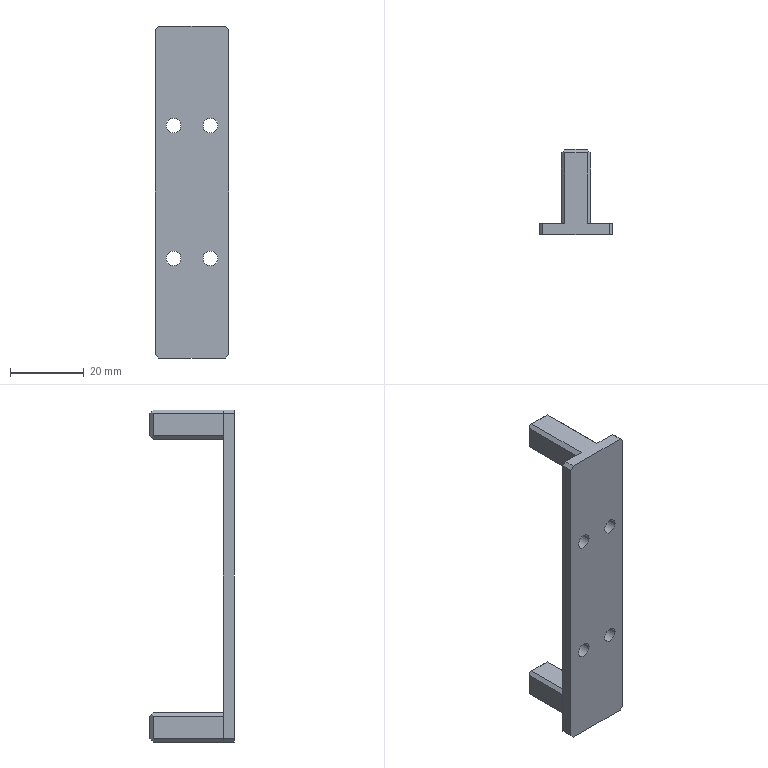Part | STEP file | Guide wheel mechanism revised.sldasm-Part-383 | 1 solid | 42 faces | box 20 x 23 x 90 mm | volume 7697 mm3 | plane 34 | cylinder 8 | commonest cylinder face diameters 4 x8
STEP:
#1=CARTESIAN_POINT('',(3.,-1.5,18.));
#2=VERTEX_POINT('',#1);
#3=CARTESIAN_POINT('',(7.,-1.5,18.));
#4=VERTEX_POINT('',#3);
#5=CARTESIAN_POINT('',(5.,-1.5,18.));
#6=DIRECTION('',(0.,-1.,0.));
#7=DIRECTION('',(-1.,0.,0.));
#8=AXIS2_PLACEMENT_3D('',#5,#6,#7);
#9=CIRCLE('',#8,2.);
#10=EDGE_CURVE('',#2,#4,#9,.T.);
#11=ORIENTED_EDGE('',*,*,#10,.T.);
#12=CARTESIAN_POINT('',(7.,1.5,18.));
#13=VERTEX_POINT('',#12);
#14=CARTESIAN_POINT('',(7.,-1.501,18.));
#15=DIRECTION('',(0.,1.,0.));
#16=VECTOR('',#15,1000.);
#17=LINE('',#14,#16);
#18=EDGE_CURVE('',#4,#13,#17,.T.);
#19=ORIENTED_EDGE('',*,*,#18,.T.);
#20=CARTESIAN_POINT('',(3.,1.5,18.));
#21=VERTEX_POINT('',#20);
#22=CARTESIAN_POINT('',(5.,1.5,18.));
#23=DIRECTION('',(0.,1.,0.));
#24=DIRECTION('',(-1.,0.,0.));
#25=AXIS2_PLACEMENT_3D('',#22,#23,#24);
#26=CIRCLE('',#25,2.);
#27=EDGE_CURVE('',#13,#21,#26,.T.);
#28=ORIENTED_EDGE('',*,*,#27,.T.);
#29=CARTESIAN_POINT('',(3.,-1.501,18.));
#30=DIRECTION('',(0.,1.,0.));
#31=VECTOR('',#30,1000.);
#32=LINE('',#29,#31);
#33=EDGE_CURVE('',#2,#21,#32,.T.);
#34=ORIENTED_EDGE('',*,*,#33,.F.);
#35=EDGE_LOOP('',(#11,#19,#28,#34));
#36=FACE_OUTER_BOUND('',#35,.T.);
#37=CARTESIAN_POINT('',(5.,-1.501,18.));
#38=DIRECTION('',(0.,1.,0.));
#39=DIRECTION('',(-1.,0.,0.));
#40=AXIS2_PLACEMENT_3D('',#37,#38,#39);
#41=CYLINDRICAL_SURFACE('',#40,2.);
#42=ADVANCED_FACE('',(#36),#41,.F.);
#43=CARTESIAN_POINT('',(-7.,-1.5,18.));
#44=VERTEX_POINT('',#43);
#45=CARTESIAN_POINT('',(-3.,-1.5,18.));
#46=VERTEX_POINT('',#45);
#47=CARTESIAN_POINT('',(-5.,-1.5,18.));
#48=DIRECTION('',(0.,-1.,0.));
#49=DIRECTION('',(-1.,0.,0.));
#50=AXIS2_PLACEMENT_3D('',#47,#48,#49);
#51=CIRCLE('',#50,2.);
#52=EDGE_CURVE('',#44,#46,#51,.T.);
#53=ORIENTED_EDGE('',*,*,#52,.T.);
#54=CARTESIAN_POINT('',(-3.,1.5,18.));
#55=VERTEX_POINT('',#54);
#56=CARTESIAN_POINT('',(-3.,-1.501,18.));
#57=DIRECTION('',(0.,1.,0.));
#58=VECTOR('',#57,1000.);
#59=LINE('',#56,#58);
#60=EDGE_CURVE('',#46,#55,#59,.T.);
#61=ORIENTED_EDGE('',*,*,#60,.T.);
#62=CARTESIAN_POINT('',(-7.,1.5,18.));
#63=VERTEX_POINT('',#62);
#64=CARTESIAN_POINT('',(-5.,1.5,18.));
#65=DIRECTION('',(0.,1.,0.));
#66=DIRECTION('',(-1.,0.,0.));
#67=AXIS2_PLACEMENT_3D('',#64,#65,#66);
#68=CIRCLE('',#67,2.);
#69=EDGE_CURVE('',#55,#63,#68,.T.);
#70=ORIENTED_EDGE('',*,*,#69,.T.);
#71=CARTESIAN_POINT('',(-7.,-1.501,18.));
#72=DIRECTION('',(0.,1.,0.));
#73=VECTOR('',#72,1000.);
#74=LINE('',#71,#73);
#75=EDGE_CURVE('',#44,#63,#74,.T.);
#76=ORIENTED_EDGE('',*,*,#75,.F.);
#77=EDGE_LOOP('',(#53,#61,#70,#76));
#78=FACE_OUTER_BOUND('',#77,.T.);
#79=CARTESIAN_POINT('',(-5.,-1.501,18.));
#80=DIRECTION('',(0.,1.,0.));
#81=DIRECTION('',(-1.,0.,0.));
#82=AXIS2_PLACEMENT_3D('',#79,#80,#81);
#83=CYLINDRICAL_SURFACE('',#82,2.);
#84=ADVANCED_FACE('',(#78),#83,.F.);
#85=CARTESIAN_POINT('',(3.,-1.5,-18.));
#86=VERTEX_POINT('',#85);
#87=CARTESIAN_POINT('',(7.,-1.5,-18.));
#88=VERTEX_POINT('',#87);
#89=CARTESIAN_POINT('',(5.,-1.5,-18.));
#90=DIRECTION('',(0.,-1.,0.));
#91=DIRECTION('',(-1.,0.,0.));
#92=AXIS2_PLACEMENT_3D('',#89,#90,#91);
#93=CIRCLE('',#92,2.);
#94=EDGE_CURVE('',#86,#88,#93,.T.);
#95=ORIENTED_EDGE('',*,*,#94,.T.);
#96=CARTESIAN_POINT('',(7.,1.5,-18.));
#97=VERTEX_POINT('',#96);
#98=CARTESIAN_POINT('',(7.,-1.501,-18.));
#99=DIRECTION('',(0.,1.,0.));
#100=VECTOR('',#99,1000.);
#101=LINE('',#98,#100);
#102=EDGE_CURVE('',#88,#97,#101,.T.);
#103=ORIENTED_EDGE('',*,*,#102,.T.);
#104=CARTESIAN_POINT('',(3.,1.5,-18.));
#105=VERTEX_POINT('',#104);
#106=CARTESIAN_POINT('',(5.,1.5,-18.));
#107=DIRECTION('',(0.,1.,0.));
#108=DIRECTION('',(-1.,0.,0.));
#109=AXIS2_PLACEMENT_3D('',#106,#107,#108);
#110=CIRCLE('',#109,2.);
#111=EDGE_CURVE('',#97,#105,#110,.T.);
#112=ORIENTED_EDGE('',*,*,#111,.T.);
#113=CARTESIAN_POINT('',(3.,-1.501,-18.));
#114=DIRECTION('',(0.,1.,0.));
#115=VECTOR('',#114,1000.);
#116=LINE('',#113,#115);
#117=EDGE_CURVE('',#86,#105,#116,.T.);
#118=ORIENTED_EDGE('',*,*,#117,.F.);
#119=EDGE_LOOP('',(#95,#103,#112,#118));
#120=FACE_OUTER_BOUND('',#119,.T.);
#121=CARTESIAN_POINT('',(5.,-1.501,-18.));
#122=DIRECTION('',(0.,1.,0.));
#123=DIRECTION('',(-1.,0.,0.));
#124=AXIS2_PLACEMENT_3D('',#121,#122,#123);
#125=CYLINDRICAL_SURFACE('',#124,2.);
#126=ADVANCED_FACE('',(#120),#125,.F.);
#127=CARTESIAN_POINT('',(-7.,-1.5,-18.));
#128=VERTEX_POINT('',#127);
#129=CARTESIAN_POINT('',(-3.,-1.5,-18.));
#130=VERTEX_POINT('',#129);
#131=CARTESIAN_POINT('',(-5.,-1.5,-18.));
#132=DIRECTION('',(0.,-1.,0.));
#133=DIRECTION('',(-1.,0.,0.));
#134=AXIS2_PLACEMENT_3D('',#131,#132,#133);
#135=CIRCLE('',#134,2.);
#136=EDGE_CURVE('',#128,#130,#135,.T.);
#137=ORIENTED_EDGE('',*,*,#136,.T.);
#138=CARTESIAN_POINT('',(-3.,1.5,-18.));
#139=VERTEX_POINT('',#138);
#140=CARTESIAN_POINT('',(-3.,-1.501,-18.));
#141=DIRECTION('',(0.,1.,0.));
#142=VECTOR('',#141,1000.);
#143=LINE('',#140,#142);
#144=EDGE_CURVE('',#130,#139,#143,.T.);
#145=ORIENTED_EDGE('',*,*,#144,.T.);
#146=CARTESIAN_POINT('',(-7.,1.5,-18.));
#147=VERTEX_POINT('',#146);
#148=CARTESIAN_POINT('',(-5.,1.5,-18.));
#149=DIRECTION('',(0.,1.,0.));
#150=DIRECTION('',(-1.,0.,0.));
#151=AXIS2_PLACEMENT_3D('',#148,#149,#150);
#152=CIRCLE('',#151,2.);
#153=EDGE_CURVE('',#139,#147,#152,.T.);
#154=ORIENTED_EDGE('',*,*,#153,.T.);
#155=CARTESIAN_POINT('',(-7.,-1.501,-18.));
#156=DIRECTION('',(0.,1.,0.));
#157=VECTOR('',#156,1000.);
#158=LINE('',#155,#157);
#159=EDGE_CURVE('',#128,#147,#158,.T.);
#160=ORIENTED_EDGE('',*,*,#159,.F.);
#161=EDGE_LOOP('',(#137,#145,#154,#160));
#162=FACE_OUTER_BOUND('',#161,.T.);
#163=CARTESIAN_POINT('',(-5.,-1.501,-18.));
#164=DIRECTION('',(0.,1.,0.));
#165=DIRECTION('',(-1.,0.,0.));
#166=AXIS2_PLACEMENT_3D('',#163,#164,#165);
#167=CYLINDRICAL_SURFACE('',#166,2.);
#168=ADVANCED_FACE('',(#162),#167,.F.);
#169=CARTESIAN_POINT('',(-4.,1.5,44.));
#170=VERTEX_POINT('',#169);
#171=CARTESIAN_POINT('',(-4.,20.5,44.));
#172=VERTEX_POINT('',#171);
#173=CARTESIAN_POINT('',(-4.,20.5,44.));
#174=DIRECTION('',(0.,1.,0.));
#175=VECTOR('',#174,1000.);
#176=LINE('',#173,#175);
#177=EDGE_CURVE('',#170,#172,#176,.T.);
#178=ORIENTED_EDGE('',*,*,#177,.T.);
#179=CARTESIAN_POINT('',(-4.,20.5,38.));
#180=VERTEX_POINT('',#179);
#181=CARTESIAN_POINT('',(-4.,20.5,38.));
#182=DIRECTION('',(0.,0.,-1.));
#183=VECTOR('',#182,1000.);
#184=LINE('',#181,#183);
#185=EDGE_CURVE('',#172,#180,#184,.T.);
#186=ORIENTED_EDGE('',*,*,#185,.T.);
#187=CARTESIAN_POINT('',(-4.,1.5,38.));
#188=VERTEX_POINT('',#187);
#189=CARTESIAN_POINT('',(-4.,21.5,38.));
#190=DIRECTION('',(0.,-1.,0.));
#191=VECTOR('',#190,1000.);
#192=LINE('',#189,#191);
#193=EDGE_CURVE('',#180,#188,#192,.T.);
#194=ORIENTED_EDGE('',*,*,#193,.T.);
#195=CARTESIAN_POINT('',(-4.,1.5,45.));
#196=DIRECTION('',(0.,0.,1.));
#197=VECTOR('',#196,1000.);
#198=LINE('',#195,#197);
#199=EDGE_CURVE('',#188,#170,#198,.T.);
#200=ORIENTED_EDGE('',*,*,#199,.T.);
#201=EDGE_LOOP('',(#178,#186,#194,#200));
#202=FACE_OUTER_BOUND('',#201,.T.);
#203=CARTESIAN_POINT('',(-4.,21.5,45.));
#204=DIRECTION('',(1.,0.,0.));
#205=DIRECTION('',(0.,1.,0.));
#206=AXIS2_PLACEMENT_3D('',#203,#204,#205);
#207=PLANE('',#206);
#208=ADVANCED_FACE('',(#202),#207,.F.);
#209=CARTESIAN_POINT('',(4.,1.5,38.));
#210=VERTEX_POINT('',#209);
#211=CARTESIAN_POINT('',(4.,20.5,38.));
#212=VERTEX_POINT('',#211);
#213=CARTESIAN_POINT('',(4.,21.5,38.));
#214=DIRECTION('',(0.,1.,0.));
#215=VECTOR('',#214,1000.);
#216=LINE('',#213,#215);
#217=EDGE_CURVE('',#210,#212,#216,.T.);
#218=ORIENTED_EDGE('',*,*,#217,.T.);
#219=CARTESIAN_POINT('',(4.,20.5,44.));
#220=VERTEX_POINT('',#219);
#221=CARTESIAN_POINT('',(4.,20.5,44.));
#222=DIRECTION('',(0.,0.,1.));
#223=VECTOR('',#222,1000.);
#224=LINE('',#221,#223);
#225=EDGE_CURVE('',#212,#220,#224,.T.);
#226=ORIENTED_EDGE('',*,*,#225,.T.);
#227=CARTESIAN_POINT('',(4.,1.5,44.));
#228=VERTEX_POINT('',#227);
#229=CARTESIAN_POINT('',(4.,1.5,44.));
#230=DIRECTION('',(0.,-1.,0.));
#231=VECTOR('',#230,1000.);
#232=LINE('',#229,#231);
#233=EDGE_CURVE('',#220,#228,#232,.T.);
#234=ORIENTED_EDGE('',*,*,#233,.T.);
#235=CARTESIAN_POINT('',(4.,1.5,45.));
#236=DIRECTION('',(0.,0.,-1.));
#237=VECTOR('',#236,1000.);
#238=LINE('',#235,#237);
#239=EDGE_CURVE('',#228,#210,#238,.T.);
#240=ORIENTED_EDGE('',*,*,#239,.T.);
#241=EDGE_LOOP('',(#218,#226,#234,#240));
#242=FACE_OUTER_BOUND('',#241,.T.);
#243=CARTESIAN_POINT('',(4.,21.5,45.));
#244=DIRECTION('',(-1.,0.,0.));
#245=DIRECTION('',(0.,-1.,0.));
#246=AXIS2_PLACEMENT_3D('',#243,#244,#245);
#247=PLANE('',#246);
#248=ADVANCED_FACE('',(#242),#247,.F.);
#249=CARTESIAN_POINT('',(-3.,21.5,44.));
#250=VERTEX_POINT('',#249);
#251=CARTESIAN_POINT('',(3.,21.5,44.));
#252=VERTEX_POINT('',#251);
#253=CARTESIAN_POINT('',(0.,21.5,44.));
#254=DIRECTION('',(1.,0.,0.));
#255=VECTOR('',#254,1000.);
#256=LINE('',#253,#255);
#257=EDGE_CURVE('',#250,#252,#256,.T.);
#258=ORIENTED_EDGE('',*,*,#257,.T.);
#259=CARTESIAN_POINT('',(3.,21.5,38.));
#260=VERTEX_POINT('',#259);
#261=CARTESIAN_POINT('',(3.,21.5,38.));
#262=DIRECTION('',(0.,0.,-1.));
#263=VECTOR('',#262,1000.);
#264=LINE('',#261,#263);
#265=EDGE_CURVE('',#252,#260,#264,.T.);
#266=ORIENTED_EDGE('',*,*,#265,.T.);
#267=CARTESIAN_POINT('',(-3.,21.5,38.));
#268=VERTEX_POINT('',#267);
#269=CARTESIAN_POINT('',(-4.,21.5,38.));
#270=DIRECTION('',(-1.,0.,0.));
#271=VECTOR('',#270,1000.);
#272=LINE('',#269,#271);
#273=EDGE_CURVE('',#260,#268,#272,.T.);
#274=ORIENTED_EDGE('',*,*,#273,.T.);
#275=CARTESIAN_POINT('',(-3.,21.5,44.));
#276=DIRECTION('',(0.,0.,1.));
#277=VECTOR('',#276,1000.);
#278=LINE('',#275,#277);
#279=EDGE_CURVE('',#268,#250,#278,.T.);
#280=ORIENTED_EDGE('',*,*,#279,.T.);
#281=EDGE_LOOP('',(#258,#266,#274,#280));
#282=FACE_OUTER_BOUND('',#281,.T.);
#283=CARTESIAN_POINT('',(0.,21.5,0.));
#284=DIRECTION('',(0.,1.,0.));
#285=DIRECTION('',(-1.,0.,0.));
#286=AXIS2_PLACEMENT_3D('',#283,#284,#285);
#287=PLANE('',#286);
#288=ADVANCED_FACE('',(#282),#287,.T.);
#289=CARTESIAN_POINT('',(5.,1.5,18.));
#290=DIRECTION('',(0.,1.,0.));
#291=DIRECTION('',(-1.,0.,0.));
#292=AXIS2_PLACEMENT_3D('',#289,#290,#291);
#293=CIRCLE('',#292,2.);
#294=EDGE_CURVE('',#21,#13,#293,.T.);
#295=ORIENTED_EDGE('',*,*,#294,.F.);
#296=ORIENTED_EDGE('',*,*,#27,.F.);
#297=EDGE_LOOP('',(#295,#296));
#298=FACE_BOUND('',#297,.T.);
#299=CARTESIAN_POINT('',(-5.,1.5,18.));
#300=DIRECTION('',(0.,1.,0.));
#301=DIRECTION('',(-1.,0.,0.));
#302=AXIS2_PLACEMENT_3D('',#299,#300,#301);
#303=CIRCLE('',#302,2.);
#304=EDGE_CURVE('',#63,#55,#303,.T.);
#305=ORIENTED_EDGE('',*,*,#304,.F.);
#306=ORIENTED_EDGE('',*,*,#69,.F.);
#307=EDGE_LOOP('',(#305,#306));
#308=FACE_BOUND('',#307,.T.);
#309=CARTESIAN_POINT('',(5.,1.5,-18.));
#310=DIRECTION('',(0.,1.,0.));
#311=DIRECTION('',(-1.,0.,0.));
#312=AXIS2_PLACEMENT_3D('',#309,#310,#311);
#313=CIRCLE('',#312,2.);
#314=EDGE_CURVE('',#105,#97,#313,.T.);
#315=ORIENTED_EDGE('',*,*,#314,.F.);
#316=ORIENTED_EDGE('',*,*,#111,.F.);
#317=EDGE_LOOP('',(#315,#316));
#318=FACE_BOUND('',#317,.T.);
#319=CARTESIAN_POINT('',(-5.,1.5,-18.));
#320=DIRECTION('',(0.,1.,0.));
#321=DIRECTION('',(-1.,0.,0.));
#322=AXIS2_PLACEMENT_3D('',#319,#320,#321);
#323=CIRCLE('',#322,2.);
#324=EDGE_CURVE('',#147,#139,#323,.T.);
#325=ORIENTED_EDGE('',*,*,#324,.F.);
#326=ORIENTED_EDGE('',*,*,#153,.F.);
#327=EDGE_LOOP('',(#325,#326));
#328=FACE_BOUND('',#327,.T.);
#329=CARTESIAN_POINT('',(-3.,1.5,-45.));
#330=VERTEX_POINT('',#329);
#331=CARTESIAN_POINT('',(-9.,1.5,-45.));
#332=VERTEX_POINT('',#331);
#333=CARTESIAN_POINT('',(10.,1.5,-45.));
#334=DIRECTION('',(-1.,0.,0.));
#335=VECTOR('',#334,1000.);
#336=LINE('',#333,#335);
#337=EDGE_CURVE('',#330,#332,#336,.T.);
#338=ORIENTED_EDGE('',*,*,#337,.T.);
#339=CARTESIAN_POINT('',(-10.,1.5,-44.));
#340=VERTEX_POINT('',#339);
#341=CARTESIAN_POINT('',(-10.,1.5,-44.));
#342=DIRECTION('',(-0.7071,0.,0.7071));
#343=VECTOR('',#342,1000.);
#344=LINE('',#341,#343);
#345=EDGE_CURVE('',#332,#340,#344,.T.);
#346=ORIENTED_EDGE('',*,*,#345,.T.);
#347=CARTESIAN_POINT('',(-10.,1.5,44.));
#348=VERTEX_POINT('',#347);
#349=CARTESIAN_POINT('',(-10.,1.5,45.));
#350=DIRECTION('',(0.,0.,-1.));
#351=VECTOR('',#350,1000.);
#352=LINE('',#349,#351);
#353=EDGE_CURVE('',#348,#340,#352,.T.);
#354=ORIENTED_EDGE('',*,*,#353,.F.);
#355=CARTESIAN_POINT('',(-9.,1.5,45.));
#356=VERTEX_POINT('',#355);
#357=CARTESIAN_POINT('',(-9.,1.5,45.));
#358=DIRECTION('',(0.7071,0.,0.7071));
#359=VECTOR('',#358,1000.);
#360=LINE('',#357,#359);
#361=EDGE_CURVE('',#348,#356,#360,.T.);
#362=ORIENTED_EDGE('',*,*,#361,.T.);
#363=CARTESIAN_POINT('',(-3.,1.5,45.));
#364=VERTEX_POINT('',#363);
#365=CARTESIAN_POINT('',(10.,1.5,45.));
#366=DIRECTION('',(-1.,0.,0.));
#367=VECTOR('',#366,1000.);
#368=LINE('',#365,#367);
#369=EDGE_CURVE('',#364,#356,#368,.T.);
#370=ORIENTED_EDGE('',*,*,#369,.F.);
#371=CARTESIAN_POINT('',(3.5,1.5,51.5));
#372=DIRECTION('',(-0.7071,0.,-0.7071));
#373=VECTOR('',#372,1000.);
#374=LINE('',#371,#373);
#375=EDGE_CURVE('',#364,#170,#374,.T.);
#376=ORIENTED_EDGE('',*,*,#375,.T.);
#377=ORIENTED_EDGE('',*,*,#199,.F.);
#378=CARTESIAN_POINT('',(-3.,1.5,37.));
#379=VERTEX_POINT('',#378);
#380=CARTESIAN_POINT('',(-0.5,1.5,34.5));
#381=DIRECTION('',(0.7071,0.,-0.7071));
#382=VECTOR('',#381,1000.);
#383=LINE('',#380,#382);
#384=EDGE_CURVE('',#188,#379,#383,.T.);
#385=ORIENTED_EDGE('',*,*,#384,.T.);
#386=CARTESIAN_POINT('',(3.,1.5,37.));
#387=VERTEX_POINT('',#386);
#388=CARTESIAN_POINT('',(-10.001,1.5,37.));
#389=DIRECTION('',(1.,0.,0.));
#390=VECTOR('',#389,1000.);
#391=LINE('',#388,#390);
#392=EDGE_CURVE('',#379,#387,#391,.T.);
#393=ORIENTED_EDGE('',*,*,#392,.T.);
#394=CARTESIAN_POINT('',(10.5,1.5,44.5));
#395=DIRECTION('',(0.7071,0.,0.7071));
#396=VECTOR('',#395,1000.);
#397=LINE('',#394,#396);
#398=EDGE_CURVE('',#387,#210,#397,.T.);
#399=ORIENTED_EDGE('',*,*,#398,.T.);
#400=ORIENTED_EDGE('',*,*,#239,.F.);
#401=CARTESIAN_POINT('',(3.,1.5,45.));
#402=VERTEX_POINT('',#401);
#403=CARTESIAN_POINT('',(6.5,1.5,41.5));
#404=DIRECTION('',(-0.7071,0.,0.7071));
#405=VECTOR('',#404,1000.);
#406=LINE('',#403,#405);
#407=EDGE_CURVE('',#228,#402,#406,.T.);
#408=ORIENTED_EDGE('',*,*,#407,.T.);
#409=CARTESIAN_POINT('',(9.,1.5,45.));
#410=VERTEX_POINT('',#409);
#411=CARTESIAN_POINT('',(10.,1.5,45.));
#412=DIRECTION('',(-1.,0.,0.));
#413=VECTOR('',#412,1000.);
#414=LINE('',#411,#413);
#415=EDGE_CURVE('',#410,#402,#414,.T.);
#416=ORIENTED_EDGE('',*,*,#415,.F.);
#417=CARTESIAN_POINT('',(10.,1.5,44.));
#418=VERTEX_POINT('',#417);
#419=CARTESIAN_POINT('',(9.,1.5,45.));
#420=DIRECTION('',(0.7071,0.,-0.7071));
#421=VECTOR('',#420,1000.);
#422=LINE('',#419,#421);
#423=EDGE_CURVE('',#410,#418,#422,.T.);
#424=ORIENTED_EDGE('',*,*,#423,.T.);
#425=CARTESIAN_POINT('',(10.,1.5,-44.));
#426=VERTEX_POINT('',#425);
#427=CARTESIAN_POINT('',(10.,1.5,45.));
#428=DIRECTION('',(0.,0.,-1.));
#429=VECTOR('',#428,1000.);
#430=LINE('',#427,#429);
#431=EDGE_CURVE('',#418,#426,#430,.T.);
#432=ORIENTED_EDGE('',*,*,#431,.T.);
#433=CARTESIAN_POINT('',(9.,1.5,-45.));
#434=VERTEX_POINT('',#433);
#435=CARTESIAN_POINT('',(10.,1.5,-44.));
#436=DIRECTION('',(-0.7071,0.,-0.7071));
#437=VECTOR('',#436,1000.);
#438=LINE('',#435,#437);
#439=EDGE_CURVE('',#426,#434,#438,.T.);
#440=ORIENTED_EDGE('',*,*,#439,.T.);
#441=CARTESIAN_POINT('',(3.,1.5,-45.));
#442=VERTEX_POINT('',#441);
#443=CARTESIAN_POINT('',(10.,1.5,-45.));
#444=DIRECTION('',(-1.,0.,0.));
#445=VECTOR('',#444,1000.);
#446=LINE('',#443,#445);
#447=EDGE_CURVE('',#434,#442,#446,.T.);
#448=ORIENTED_EDGE('',*,*,#447,.T.);
#449=CARTESIAN_POINT('',(4.,1.5,-44.));
#450=VERTEX_POINT('',#449);
#451=CARTESIAN_POINT('',(51.5,1.5,3.5));
#452=DIRECTION('',(0.7071,0.,0.7071));
#453=VECTOR('',#452,1000.);
#454=LINE('',#451,#453);
#455=EDGE_CURVE('',#442,#450,#454,.T.);
#456=ORIENTED_EDGE('',*,*,#455,.T.);
#457=CARTESIAN_POINT('',(4.,1.5,-38.));
#458=VERTEX_POINT('',#457);
#459=CARTESIAN_POINT('',(4.,1.5,45.));
#460=DIRECTION('',(0.,0.,-1.));
#461=VECTOR('',#460,1000.);
#462=LINE('',#459,#461);
#463=EDGE_CURVE('',#458,#450,#462,.T.);
#464=ORIENTED_EDGE('',*,*,#463,.F.);
#465=CARTESIAN_POINT('',(3.,1.5,-37.));
#466=VERTEX_POINT('',#465);
#467=CARTESIAN_POINT('',(-34.5,1.5,0.5));
#468=DIRECTION('',(-0.7071,0.,0.7071));
#469=VECTOR('',#468,1000.);
#470=LINE('',#467,#469);
#471=EDGE_CURVE('',#458,#466,#470,.T.);
#472=ORIENTED_EDGE('',*,*,#471,.T.);
#473=CARTESIAN_POINT('',(-3.,1.5,-37.));
#474=VERTEX_POINT('',#473);
#475=CARTESIAN_POINT('',(-10.001,1.5,-37.));
#476=DIRECTION('',(1.,0.,0.));
#477=VECTOR('',#476,1000.);
#478=LINE('',#475,#477);
#479=EDGE_CURVE('',#474,#466,#478,.T.);
#480=ORIENTED_EDGE('',*,*,#479,.F.);
#481=CARTESIAN_POINT('',(-4.,1.5,-38.));
#482=VERTEX_POINT('',#481);
#483=CARTESIAN_POINT('',(44.5,1.5,10.5));
#484=DIRECTION('',(-0.7071,0.,-0.7071));
#485=VECTOR('',#484,1000.);
#486=LINE('',#483,#485);
#487=EDGE_CURVE('',#474,#482,#486,.T.);
#488=ORIENTED_EDGE('',*,*,#487,.T.);
#489=CARTESIAN_POINT('',(-4.,1.5,-44.));
#490=VERTEX_POINT('',#489);
#491=CARTESIAN_POINT('',(-4.,1.5,45.));
#492=DIRECTION('',(0.,0.,1.));
#493=VECTOR('',#492,1000.);
#494=LINE('',#491,#493);
#495=EDGE_CURVE('',#490,#482,#494,.T.);
#496=ORIENTED_EDGE('',*,*,#495,.F.);
#497=CARTESIAN_POINT('',(-41.5,1.5,-6.5));
#498=DIRECTION('',(0.7071,0.,-0.7071));
#499=VECTOR('',#498,1000.);
#500=LINE('',#497,#499);
#501=EDGE_CURVE('',#490,#330,#500,.T.);
#502=ORIENTED_EDGE('',*,*,#501,.T.);
#503=EDGE_LOOP('',(#338,#346,#354,#362,#370,#376,#377,#385,#393,#399,#400,#408,#416,#424,#432,#440,#448,#456,#464,#472,#480,#488,#496,#502));
#504=FACE_OUTER_BOUND('',#503,.T.);
#505=CARTESIAN_POINT('',(10.,1.5,45.));
#506=DIRECTION('',(0.,-1.,0.));
#507=DIRECTION('',(1.,0.,0.));
#508=AXIS2_PLACEMENT_3D('',#505,#506,#507);
#509=PLANE('',#508);
#510=ADVANCED_FACE('',(#298,#308,#318,#328,#504),#509,.F.);
#511=ORIENTED_EDGE('',*,*,#353,.T.);
#512=CARTESIAN_POINT('',(-10.,-1.5,-44.));
#513=VERTEX_POINT('',#512);
#514=CARTESIAN_POINT('',(-10.,-1.5,-44.));
#515=DIRECTION('',(0.,-1.,0.));
#516=VECTOR('',#515,1000.);
#517=LINE('',#514,#516);
#518=EDGE_CURVE('',#340,#513,#517,.T.);
#519=ORIENTED_EDGE('',*,*,#518,.T.);
#520=CARTESIAN_POINT('',(-10.,-1.5,44.));
#521=VERTEX_POINT('',#520);
#522=CARTESIAN_POINT('',(-10.,-1.5,45.));
#523=DIRECTION('',(0.,0.,-1.));
#524=VECTOR('',#523,1000.);
#525=LINE('',#522,#524);
#526=EDGE_CURVE('',#521,#513,#525,.T.);
#527=ORIENTED_EDGE('',*,*,#526,.F.);
#528=CARTESIAN_POINT('',(-10.,1.5,44.));
#529=DIRECTION('',(0.,1.,0.));
#530=VECTOR('',#529,1000.);
#531=LINE('',#528,#530);
#532=EDGE_CURVE('',#521,#348,#531,.T.);
#533=ORIENTED_EDGE('',*,*,#532,.T.);
#534=EDGE_LOOP('',(#511,#519,#527,#533));
#535=FACE_OUTER_BOUND('',#534,.T.);
#536=CARTESIAN_POINT('',(-10.,-1.5,45.));
#537=DIRECTION('',(1.,0.,0.));
#538=DIRECTION('',(0.,0.,-1.));
#539=AXIS2_PLACEMENT_3D('',#536,#537,#538);
#540=PLANE('',#539);
#541=ADVANCED_FACE('',(#535),#540,.F.);
#542=ORIENTED_EDGE('',*,*,#10,.F.);
#543=CARTESIAN_POINT('',(5.,-1.5,18.));
#544=DIRECTION('',(0.,-1.,0.));
#545=DIRECTION('',(-1.,0.,0.));
#546=AXIS2_PLACEMENT_3D('',#543,#544,#545);
#547=CIRCLE('',#546,2.);
#548=EDGE_CURVE('',#4,#2,#547,.T.);
#549=ORIENTED_EDGE('',*,*,#548,.F.);
#550=EDGE_LOOP('',(#542,#549));
#551=FACE_BOUND('',#550,.T.);
#552=ORIENTED_EDGE('',*,*,#52,.F.);
#553=CARTESIAN_POINT('',(-5.,-1.5,18.));
#554=DIRECTION('',(0.,-1.,0.));
#555=DIRECTION('',(-1.,0.,0.));
#556=AXIS2_PLACEMENT_3D('',#553,#554,#555);
#557=CIRCLE('',#556,2.);
#558=EDGE_CURVE('',#46,#44,#557,.T.);
#559=ORIENTED_EDGE('',*,*,#558,.F.);
#560=EDGE_LOOP('',(#552,#559));
#561=FACE_BOUND('',#560,.T.);
#562=ORIENTED_EDGE('',*,*,#94,.F.);
#563=CARTESIAN_POINT('',(5.,-1.5,-18.));
#564=DIRECTION('',(0.,-1.,0.));
#565=DIRECTION('',(-1.,0.,0.));
#566=AXIS2_PLACEMENT_3D('',#563,#564,#565);
#567=CIRCLE('',#566,2.);
#568=EDGE_CURVE('',#88,#86,#567,.T.);
#569=ORIENTED_EDGE('',*,*,#568,.F.);
#570=EDGE_LOOP('',(#562,#569));
#571=FACE_BOUND('',#570,.T.);
#572=ORIENTED_EDGE('',*,*,#136,.F.);
#573=CARTESIAN_POINT('',(-5.,-1.5,-18.));
#574=DIRECTION('',(0.,-1.,0.));
#575=DIRECTION('',(-1.,0.,0.));
#576=AXIS2_PLACEMENT_3D('',#573,#574,#575);
#577=CIRCLE('',#576,2.);
#578=EDGE_CURVE('',#130,#128,#577,.T.);
#579=ORIENTED_EDGE('',*,*,#578,.F.);
#580=EDGE_LOOP('',(#572,#579));
#581=FACE_BOUND('',#580,.T.);
#582=ORIENTED_EDGE('',*,*,#526,.T.);
#583=CARTESIAN_POINT('',(-9.,-1.5,-45.));
#584=VERTEX_POINT('',#583);
#585=CARTESIAN_POINT('',(-10.,-1.5,-44.));
#586=DIRECTION('',(0.7071,0.,-0.7071));
#587=VECTOR('',#586,1000.);
#588=LINE('',#585,#587);
#589=EDGE_CURVE('',#513,#584,#588,.T.);
#590=ORIENTED_EDGE('',*,*,#589,.T.);
#591=CARTESIAN_POINT('',(9.,-1.5,-45.));
#592=VERTEX_POINT('',#591);
#593=CARTESIAN_POINT('',(10.,-1.5,-45.));
#594=DIRECTION('',(1.,0.,0.));
#595=VECTOR('',#594,1000.);
#596=LINE('',#593,#595);
#597=EDGE_CURVE('',#584,#592,#596,.T.);
#598=ORIENTED_EDGE('',*,*,#597,.T.);
#599=CARTESIAN_POINT('',(10.,-1.5,-44.));
#600=VERTEX_POINT('',#599);
#601=CARTESIAN_POINT('',(10.,-1.5,-44.));
#602=DIRECTION('',(0.7071,0.,0.7071));
#603=VECTOR('',#602,1000.);
#604=LINE('',#601,#603);
#605=EDGE_CURVE('',#592,#600,#604,.T.);
#606=ORIENTED_EDGE('',*,*,#605,.T.);
#607=CARTESIAN_POINT('',(10.,-1.5,44.));
#608=VERTEX_POINT('',#607);
#609=CARTESIAN_POINT('',(10.,-1.5,45.));
#610=DIRECTION('',(0.,0.,-1.));
#611=VECTOR('',#610,1000.);
#612=LINE('',#609,#611);
#613=EDGE_CURVE('',#608,#600,#612,.T.);
#614=ORIENTED_EDGE('',*,*,#613,.F.);
#615=CARTESIAN_POINT('',(9.,-1.5,45.));
#616=VERTEX_POINT('',#615);
#617=CARTESIAN_POINT('',(9.,-1.5,45.));
#618=DIRECTION('',(-0.7071,0.,0.7071));
#619=VECTOR('',#618,1000.);
#620=LINE('',#617,#619);
#621=EDGE_CURVE('',#608,#616,#620,.T.);
#622=ORIENTED_EDGE('',*,*,#621,.T.);
#623=CARTESIAN_POINT('',(-9.,-1.5,45.));
#624=VERTEX_POINT('',#623);
#625=CARTESIAN_POINT('',(10.,-1.5,45.));
#626=DIRECTION('',(1.,0.,0.));
#627=VECTOR('',#626,1000.);
#628=LINE('',#625,#627);
#629=EDGE_CURVE('',#624,#616,#628,.T.);
#630=ORIENTED_EDGE('',*,*,#629,.F.);
#631=CARTESIAN_POINT('',(-9.,-1.5,45.));
#632=DIRECTION('',(-0.7071,0.,-0.7071));
#633=VECTOR('',#632,1000.);
#634=LINE('',#631,#633);
#635=EDGE_CURVE('',#624,#521,#634,.T.);
#636=ORIENTED_EDGE('',*,*,#635,.T.);
#637=EDGE_LOOP('',(#582,#590,#598,#606,#614,#622,#630,#636));
#638=FACE_OUTER_BOUND('',#637,.T.);
#639=CARTESIAN_POINT('',(10.,-1.5,45.));
#640=DIRECTION('',(0.,1.,0.));
#641=DIRECTION('',(-1.,0.,0.));
#642=AXIS2_PLACEMENT_3D('',#639,#640,#641);
#643=PLANE('',#642);
#644=ADVANCED_FACE('',(#551,#561,#571,#581,#638),#643,.F.);
#645=ORIENTED_EDGE('',*,*,#613,.T.);
#646=CARTESIAN_POINT('',(10.,-1.5,-44.));
#647=DIRECTION('',(0.,1.,0.));
#648=VECTOR('',#647,1000.);
#649=LINE('',#646,#648);
#650=EDGE_CURVE('',#600,#426,#649,.T.);
#651=ORIENTED_EDGE('',*,*,#650,.T.);
#652=ORIENTED_EDGE('',*,*,#431,.F.);
#653=CARTESIAN_POINT('',(10.,-1.5,44.));
#654=DIRECTION('',(0.,-1.,0.));
#655=VECTOR('',#654,1000.);
#656=LINE('',#653,#655);
#657=EDGE_CURVE('',#418,#608,#656,.T.);
#658=ORIENTED_EDGE('',*,*,#657,.T.);
#659=EDGE_LOOP('',(#645,#651,#652,#658));
#660=FACE_OUTER_BOUND('',#659,.T.);
#661=CARTESIAN_POINT('',(10.,-1.5,45.));
#662=DIRECTION('',(-1.,0.,0.));
#663=DIRECTION('',(0.,0.,1.));
#664=AXIS2_PLACEMENT_3D('',#661,#662,#663);
#665=PLANE('',#664);
#666=ADVANCED_FACE('',(#660),#665,.F.);
#667=CARTESIAN_POINT('',(3.,20.5,45.));
#668=VERTEX_POINT('',#667);
#669=CARTESIAN_POINT('',(-3.,20.5,45.));
#670=VERTEX_POINT('',#669);
#671=CARTESIAN_POINT('',(0.,20.5,45.));
#672=DIRECTION('',(-1.,0.,0.));
#673=VECTOR('',#672,1000.);
#674=LINE('',#671,#673);
#675=EDGE_CURVE('',#668,#670,#674,.T.);
#676=ORIENTED_EDGE('',*,*,#675,.T.);
#677=CARTESIAN_POINT('',(-3.,1.5,45.));
#678=DIRECTION('',(0.,-1.,0.));
#679=VECTOR('',#678,1000.);
#680=LINE('',#677,#679);
#681=EDGE_CURVE('',#670,#364,#680,.T.);
#682=ORIENTED_EDGE('',*,*,#681,.T.);
#683=ORIENTED_EDGE('',*,*,#369,.T.);
#684=CARTESIAN_POINT('',(-9.,-1.5,45.));
#685=DIRECTION('',(0.,-1.,0.));
#686=VECTOR('',#685,1000.);
#687=LINE('',#684,#686);
#688=EDGE_CURVE('',#356,#624,#687,.T.);
#689=ORIENTED_EDGE('',*,*,#688,.T.);
#690=ORIENTED_EDGE('',*,*,#629,.T.);
#691=CARTESIAN_POINT('',(9.,1.5,45.));
#692=DIRECTION('',(0.,1.,0.));
#693=VECTOR('',#692,1000.);
#694=LINE('',#691,#693);
#695=EDGE_CURVE('',#616,#410,#694,.T.);
#696=ORIENTED_EDGE('',*,*,#695,.T.);
#697=ORIENTED_EDGE('',*,*,#415,.T.);
#698=CARTESIAN_POINT('',(3.,20.5,45.));
#699=DIRECTION('',(0.,1.,0.));
#700=VECTOR('',#699,1000.);
#701=LINE('',#698,#700);
#702=EDGE_CURVE('',#402,#668,#701,.T.);
#703=ORIENTED_EDGE('',*,*,#702,.T.);
#704=EDGE_LOOP('',(#676,#682,#683,#689,#690,#696,#697,#703));
#705=FACE_OUTER_BOUND('',#704,.T.);
#706=CARTESIAN_POINT('',(0.,0.,45.));
#707=DIRECTION('',(0.,0.,1.));
#708=DIRECTION('',(1.,0.,0.));
#709=AXIS2_PLACEMENT_3D('',#706,#707,#708);
#710=PLANE('',#709);
#711=ADVANCED_FACE('',(#705),#710,.T.);
#712=CARTESIAN_POINT('',(-3.,20.5,-45.));
#713=VERTEX_POINT('',#712);
#714=CARTESIAN_POINT('',(3.,20.5,-45.));
#715=VERTEX_POINT('',#714);
#716=CARTESIAN_POINT('',(4.,20.5,-45.));
#717=DIRECTION('',(1.,0.,0.));
#718=VECTOR('',#717,1000.);
#719=LINE('',#716,#718);
#720=EDGE_CURVE('',#713,#715,#719,.T.);
#721=ORIENTED_EDGE('',*,*,#720,.T.);
#722=CARTESIAN_POINT('',(3.,0.,-45.));
#723=DIRECTION('',(0.,-1.,0.));
#724=VECTOR('',#723,1000.);
#725=LINE('',#722,#724);
#726=EDGE_CURVE('',#715,#442,#725,.T.);
#727=ORIENTED_EDGE('',*,*,#726,.T.);
#728=ORIENTED_EDGE('',*,*,#447,.F.);
#729=CARTESIAN_POINT('',(9.,0.,-45.));
#730=DIRECTION('',(0.,-1.,0.));
#731=VECTOR('',#730,1000.);
#732=LINE('',#729,#731);
#733=EDGE_CURVE('',#434,#592,#732,.T.);
#734=ORIENTED_EDGE('',*,*,#733,.T.);
#735=ORIENTED_EDGE('',*,*,#597,.F.);
#736=CARTESIAN_POINT('',(-9.,0.,-45.));
#737=DIRECTION('',(0.,1.,0.));
#738=VECTOR('',#737,1000.);
#739=LINE('',#736,#738);
#740=EDGE_CURVE('',#584,#332,#739,.T.);
#741=ORIENTED_EDGE('',*,*,#740,.T.);
#742=ORIENTED_EDGE('',*,*,#337,.F.);
#743=CARTESIAN_POINT('',(-3.,0.,-45.));
#744=DIRECTION('',(0.,1.,0.));
#745=VECTOR('',#744,1000.);
#746=LINE('',#743,#745);
#747=EDGE_CURVE('',#330,#713,#746,.T.);
#748=ORIENTED_EDGE('',*,*,#747,.T.);
#749=EDGE_LOOP('',(#721,#727,#728,#734,#735,#741,#742,#748));
#750=FACE_OUTER_BOUND('',#749,.T.);
#751=CARTESIAN_POINT('',(0.,0.,-45.));
#752=DIRECTION('',(0.,0.,1.));
#753=DIRECTION('',(1.,0.,0.));
#754=AXIS2_PLACEMENT_3D('',#751,#752,#753);
#755=PLANE('',#754);
#756=ADVANCED_FACE('',(#750),#755,.F.);
#757=CARTESIAN_POINT('',(-4.,20.5,-38.));
#758=VERTEX_POINT('',#757);
#759=CARTESIAN_POINT('',(-4.,21.5,-38.));
#760=DIRECTION('',(0.,1.,0.));
#761=VECTOR('',#760,1000.);
#762=LINE('',#759,#761);
#763=EDGE_CURVE('',#482,#758,#762,.T.);
#764=ORIENTED_EDGE('',*,*,#763,.T.);
#765=CARTESIAN_POINT('',(-4.,20.5,-44.));
#766=VERTEX_POINT('',#765);
#767=CARTESIAN_POINT('',(-4.,20.5,-44.));
#768=DIRECTION('',(0.,0.,-1.));
#769=VECTOR('',#768,1000.);
#770=LINE('',#767,#769);
#771=EDGE_CURVE('',#758,#766,#770,.T.);
#772=ORIENTED_EDGE('',*,*,#771,.T.);
#773=CARTESIAN_POINT('',(-4.,21.5,-44.));
#774=DIRECTION('',(0.,-1.,0.));
#775=VECTOR('',#774,1000.);
#776=LINE('',#773,#775);
#777=EDGE_CURVE('',#766,#490,#776,.T.);
#778=ORIENTED_EDGE('',*,*,#777,.T.);
#779=ORIENTED_EDGE('',*,*,#495,.T.);
#780=EDGE_LOOP('',(#764,#772,#778,#779));
#781=FACE_OUTER_BOUND('',#780,.T.);
#782=CARTESIAN_POINT('',(-4.,21.5,45.));
#783=DIRECTION('',(1.,0.,0.));
#784=DIRECTION('',(0.,1.,0.));
#785=AXIS2_PLACEMENT_3D('',#782,#783,#784);
#786=PLANE('',#785);
#787=ADVANCED_FACE('',(#781),#786,.F.);
#788=CARTESIAN_POINT('',(4.,20.5,-44.));
#789=VERTEX_POINT('',#788);
#790=CARTESIAN_POINT('',(4.,21.5,-44.));
#791=DIRECTION('',(0.,1.,0.));
#792=VECTOR('',#791,1000.);
#793=LINE('',#790,#792);
#794=EDGE_CURVE('',#450,#789,#793,.T.);
#795=ORIENTED_EDGE('',*,*,#794,.T.);
#796=CARTESIAN_POINT('',(4.,20.5,-38.));
#797=VERTEX_POINT('',#796);
#798=CARTESIAN_POINT('',(4.,20.5,-38.));
#799=DIRECTION('',(0.,0.,1.));
#800=VECTOR('',#799,1000.);
#801=LINE('',#798,#800);
#802=EDGE_CURVE('',#789,#797,#801,.T.);
#803=ORIENTED_EDGE('',*,*,#802,.T.);
#804=CARTESIAN_POINT('',(4.,21.5,-38.));
#805=DIRECTION('',(0.,-1.,0.));
#806=VECTOR('',#805,1000.);
#807=LINE('',#804,#806);
#808=EDGE_CURVE('',#797,#458,#807,.T.);
#809=ORIENTED_EDGE('',*,*,#808,.T.);
#810=ORIENTED_EDGE('',*,*,#463,.T.);
#811=EDGE_LOOP('',(#795,#803,#809,#810));
#812=FACE_OUTER_BOUND('',#811,.T.);
#813=CARTESIAN_POINT('',(4.,21.5,45.));
#814=DIRECTION('',(-1.,0.,0.));
#815=DIRECTION('',(0.,-1.,0.));
#816=AXIS2_PLACEMENT_3D('',#813,#814,#815);
#817=PLANE('',#816);
#818=ADVANCED_FACE('',(#812),#817,.F.);
#819=CARTESIAN_POINT('',(-3.,21.5,-38.));
#820=VERTEX_POINT('',#819);
#821=CARTESIAN_POINT('',(3.,21.5,-38.));
#822=VERTEX_POINT('',#821);
#823=CARTESIAN_POINT('',(4.,21.5,-38.));
#824=DIRECTION('',(1.,0.,0.));
#825=VECTOR('',#824,1000.);
#826=LINE('',#823,#825);
#827=EDGE_CURVE('',#820,#822,#826,.T.);
#828=ORIENTED_EDGE('',*,*,#827,.T.);
#829=CARTESIAN_POINT('',(3.,21.5,-44.));
#830=VERTEX_POINT('',#829);
#831=CARTESIAN_POINT('',(3.,21.5,-44.));
#832=DIRECTION('',(0.,0.,-1.));
#833=VECTOR('',#832,1000.);
#834=LINE('',#831,#833);
#835=EDGE_CURVE('',#822,#830,#834,.T.);
#836=ORIENTED_EDGE('',*,*,#835,.T.);
#837=CARTESIAN_POINT('',(-3.,21.5,-44.));
#838=VERTEX_POINT('',#837);
#839=CARTESIAN_POINT('',(-4.,21.5,-44.));
#840=DIRECTION('',(-1.,0.,0.));
#841=VECTOR('',#840,1000.);
#842=LINE('',#839,#841);
#843=EDGE_CURVE('',#830,#838,#842,.T.);
#844=ORIENTED_EDGE('',*,*,#843,.T.);
#845=CARTESIAN_POINT('',(-3.,21.5,-38.));
#846=DIRECTION('',(0.,0.,1.));
#847=VECTOR('',#846,1000.);
#848=LINE('',#845,#847);
#849=EDGE_CURVE('',#838,#820,#848,.T.);
#850=ORIENTED_EDGE('',*,*,#849,.T.);
#851=EDGE_LOOP('',(#828,#836,#844,#850));
#852=FACE_OUTER_BOUND('',#851,.T.);
#853=CARTESIAN_POINT('',(0.,21.5,0.));
#854=DIRECTION('',(0.,1.,0.));
#855=DIRECTION('',(-1.,0.,0.));
#856=AXIS2_PLACEMENT_3D('',#853,#854,#855);
#857=PLANE('',#856);
#858=ADVANCED_FACE('',(#852),#857,.T.);
#859=ORIENTED_EDGE('',*,*,#392,.F.);
#860=CARTESIAN_POINT('',(-3.,20.5,37.));
#861=VERTEX_POINT('',#860);
#862=CARTESIAN_POINT('',(-3.,21.5,37.));
#863=DIRECTION('',(0.,1.,0.));
#864=VECTOR('',#863,1000.);
#865=LINE('',#862,#864);
#866=EDGE_CURVE('',#379,#861,#865,.T.);
#867=ORIENTED_EDGE('',*,*,#866,.T.);
#868=CARTESIAN_POINT('',(3.,20.5,37.));
#869=VERTEX_POINT('',#868);
#870=CARTESIAN_POINT('',(4.,20.5,37.));
#871=DIRECTION('',(1.,0.,0.));
#872=VECTOR('',#871,1000.);
#873=LINE('',#870,#872);
#874=EDGE_CURVE('',#861,#869,#873,.T.);
#875=ORIENTED_EDGE('',*,*,#874,.T.);
#876=CARTESIAN_POINT('',(3.,21.5,37.));
#877=DIRECTION('',(0.,-1.,0.));
#878=VECTOR('',#877,1000.);
#879=LINE('',#876,#878);
#880=EDGE_CURVE('',#869,#387,#879,.T.);
#881=ORIENTED_EDGE('',*,*,#880,.T.);
#882=EDGE_LOOP('',(#859,#867,#875,#881));
#883=FACE_OUTER_BOUND('',#882,.T.);
#884=CARTESIAN_POINT('',(-10.001,21.5,37.));
#885=DIRECTION('',(0.,0.,1.));
#886=DIRECTION('',(1.,0.,0.));
#887=AXIS2_PLACEMENT_3D('',#884,#885,#886);
#888=PLANE('',#887);
#889=ADVANCED_FACE('',(#883),#888,.F.);
#890=ORIENTED_EDGE('',*,*,#479,.T.);
#891=CARTESIAN_POINT('',(3.,20.5,-37.));
#892=VERTEX_POINT('',#891);
#893=CARTESIAN_POINT('',(3.,21.5,-37.));
#894=DIRECTION('',(0.,1.,0.));
#895=VECTOR('',#894,1000.);
#896=LINE('',#893,#895);
#897=EDGE_CURVE('',#466,#892,#896,.T.);
#898=ORIENTED_EDGE('',*,*,#897,.T.);
#899=CARTESIAN_POINT('',(-3.,20.5,-37.));
#900=VERTEX_POINT('',#899);
#901=CARTESIAN_POINT('',(-4.,20.5,-37.));
#902=DIRECTION('',(-1.,0.,0.));
#903=VECTOR('',#902,1000.);
#904=LINE('',#901,#903);
#905=EDGE_CURVE('',#892,#900,#904,.T.);
#906=ORIENTED_EDGE('',*,*,#905,.T.);
#907=CARTESIAN_POINT('',(-3.,21.5,-37.));
#908=DIRECTION('',(0.,-1.,0.));
#909=VECTOR('',#908,1000.);
#910=LINE('',#907,#909);
#911=EDGE_CURVE('',#900,#474,#910,.T.);
#912=ORIENTED_EDGE('',*,*,#911,.T.);
#913=EDGE_LOOP('',(#890,#898,#906,#912));
#914=FACE_OUTER_BOUND('',#913,.T.);
#915=CARTESIAN_POINT('',(-10.001,21.5,-37.));
#916=DIRECTION('',(0.,0.,-1.));
#917=DIRECTION('',(-1.,0.,0.));
#918=AXIS2_PLACEMENT_3D('',#915,#916,#917);
#919=PLANE('',#918);
#920=ADVANCED_FACE('',(#914),#919,.F.);
#921=ORIENTED_EDGE('',*,*,#843,.F.);
#922=CARTESIAN_POINT('',(3.5,21.,-44.5));
#923=VERTEX_POINT('',#922);
#924=CARTESIAN_POINT('',(2.,22.5,-43.));
#925=DIRECTION('',(0.5774,-0.5774,-0.5774));
#926=VECTOR('',#925,1000.);
#927=LINE('',#924,#926);
#928=EDGE_CURVE('',#830,#923,#927,.T.);
#929=ORIENTED_EDGE('',*,*,#928,.T.);
#930=CARTESIAN_POINT('',(2.667,20.167,-45.333));
#931=DIRECTION('',(-0.5774,-0.5774,-0.5774));
#932=VECTOR('',#931,1000.);
#933=LINE('',#930,#932);
#934=EDGE_CURVE('',#923,#715,#933,.T.);
#935=ORIENTED_EDGE('',*,*,#934,.T.);
#936=ORIENTED_EDGE('',*,*,#720,.F.);
#937=CARTESIAN_POINT('',(-3.5,21.,-44.5));
#938=VERTEX_POINT('',#937);
#939=CARTESIAN_POINT('',(-2.667,20.167,-45.333));
#940=DIRECTION('',(-0.5774,0.5774,0.5774));
#941=VECTOR('',#940,1000.);
#942=LINE('',#939,#941);
#943=EDGE_CURVE('',#713,#938,#942,.T.);
#944=ORIENTED_EDGE('',*,*,#943,.T.);
#945=CARTESIAN_POINT('',(-2.,22.5,-43.));
#946=DIRECTION('',(0.5774,0.5774,0.5774));
#947=VECTOR('',#946,1000.);
#948=LINE('',#945,#947);
#949=EDGE_CURVE('',#938,#838,#948,.T.);
#950=ORIENTED_EDGE('',*,*,#949,.T.);
#951=EDGE_LOOP('',(#921,#929,#935,#936,#944,#950));
#952=FACE_OUTER_BOUND('',#951,.T.);
#953=CARTESIAN_POINT('',(0.,21.5,-44.));
#954=DIRECTION('',(0.,0.7071,-0.7071));
#955=DIRECTION('',(1.,0.,0.));
#956=AXIS2_PLACEMENT_3D('',#953,#954,#955);
#957=PLANE('',#956);
#958=ADVANCED_FACE('',(#952),#957,.T.);
#959=CARTESIAN_POINT('',(3.5,21.,-37.5));
#960=VERTEX_POINT('',#959);
#961=CARTESIAN_POINT('',(2.667,20.167,-36.667));
#962=DIRECTION('',(0.5774,0.5774,-0.5774));
#963=VECTOR('',#962,1000.);
#964=LINE('',#961,#963);
#965=EDGE_CURVE('',#892,#960,#964,.T.);
#966=ORIENTED_EDGE('',*,*,#965,.T.);
#967=CARTESIAN_POINT('',(2.,22.5,-39.));
#968=DIRECTION('',(-0.5774,0.5774,-0.5774));
#969=VECTOR('',#968,1000.);
#970=LINE('',#967,#969);
#971=EDGE_CURVE('',#960,#822,#970,.T.);
#972=ORIENTED_EDGE('',*,*,#971,.T.);
#973=ORIENTED_EDGE('',*,*,#827,.F.);
#974=CARTESIAN_POINT('',(-3.5,21.,-37.5));
#975=VERTEX_POINT('',#974);
#976=CARTESIAN_POINT('',(-2.,22.5,-39.));
#977=DIRECTION('',(-0.5774,-0.5774,0.5774));
#978=VECTOR('',#977,1000.);
#979=LINE('',#976,#978);
#980=EDGE_CURVE('',#820,#975,#979,.T.);
#981=ORIENTED_EDGE('',*,*,#980,.T.);
#982=CARTESIAN_POINT('',(-2.667,20.167,-36.667));
#983=DIRECTION('',(0.5774,-0.5774,0.5774));
#984=VECTOR('',#983,1000.);
#985=LINE('',#982,#984);
#986=EDGE_CURVE('',#975,#900,#985,.T.);
#987=ORIENTED_EDGE('',*,*,#986,.T.);
#988=ORIENTED_EDGE('',*,*,#905,.F.);
#989=EDGE_LOOP('',(#966,#972,#973,#981,#987,#988));
#990=FACE_OUTER_BOUND('',#989,.T.);
#991=CARTESIAN_POINT('',(0.,21.5,-38.));
#992=DIRECTION('',(0.,0.7071,0.7071));
#993=DIRECTION('',(-1.,0.,0.));
#994=AXIS2_PLACEMENT_3D('',#991,#992,#993);
#995=PLANE('',#994);
#996=ADVANCED_FACE('',(#990),#995,.T.);
#997=CARTESIAN_POINT('',(3.5,21.,44.5));
#998=VERTEX_POINT('',#997);
#999=CARTESIAN_POINT('',(2.667,20.167,45.333));
#1000=DIRECTION('',(0.5774,0.5774,-0.5774));
#1001=VECTOR('',#1000,1000.);
#1002=LINE('',#999,#1001);
#1003=EDGE_CURVE('',#668,#998,#1002,.T.);
#1004=ORIENTED_EDGE('',*,*,#1003,.T.);
#1005=CARTESIAN_POINT('',(2.,22.5,43.));
#1006=DIRECTION('',(-0.5774,0.5774,-0.5774));
#1007=VECTOR('',#1006,1000.);
#1008=LINE('',#1005,#1007);
#1009=EDGE_CURVE('',#998,#252,#1008,.T.);
#1010=ORIENTED_EDGE('',*,*,#1009,.T.);
#1011=ORIENTED_EDGE('',*,*,#257,.F.);
#1012=CARTESIAN_POINT('',(-3.5,21.,44.5));
#1013=VERTEX_POINT('',#1012);
#1014=CARTESIAN_POINT('',(-2.,22.5,43.));
#1015=DIRECTION('',(-0.5774,-0.5774,0.5774));
#1016=VECTOR('',#1015,1000.);
#1017=LINE('',#1014,#1016);
#1018=EDGE_CURVE('',#250,#1013,#1017,.T.);
#1019=ORIENTED_EDGE('',*,*,#1018,.T.);
#1020=CARTESIAN_POINT('',(-2.667,20.167,45.333));
#1021=DIRECTION('',(0.5774,-0.5774,0.5774));
#1022=VECTOR('',#1021,1000.);
#1023=LINE('',#1020,#1022);
#1024=EDGE_CURVE('',#1013,#670,#1023,.T.);
#1025=ORIENTED_EDGE('',*,*,#1024,.T.);
#1026=ORIENTED_EDGE('',*,*,#675,.F.);
#1027=EDGE_LOOP('',(#1004,#1010,#1011,#1019,#1025,#1026));
#1028=FACE_OUTER_BOUND('',#1027,.T.);
#1029=CARTESIAN_POINT('',(0.,21.5,44.));
#1030=DIRECTION('',(0.,-0.7071,-0.7071));
#1031=DIRECTION('',(1.,0.,0.));
#1032=AXIS2_PLACEMENT_3D('',#1029,#1030,#1031);
#1033=PLANE('',#1032);
#1034=ADVANCED_FACE('',(#1028),#1033,.F.);
#1035=ORIENTED_EDGE('',*,*,#273,.F.);
#1036=CARTESIAN_POINT('',(3.5,21.,37.5));
#1037=VERTEX_POINT('',#1036);
#1038=CARTESIAN_POINT('',(-0.667,25.167,41.667));
#1039=DIRECTION('',(0.5774,-0.5774,-0.5774));
#1040=VECTOR('',#1039,1000.);
#1041=LINE('',#1038,#1040);
#1042=EDGE_CURVE('',#260,#1037,#1041,.T.);
#1043=ORIENTED_EDGE('',*,*,#1042,.T.);
#1044=CARTESIAN_POINT('',(-1.334,16.166,32.666));
#1045=DIRECTION('',(-0.5774,-0.5774,-0.5774));
#1046=VECTOR('',#1045,1000.);
#1047=LINE('',#1044,#1046);
#1048=EDGE_CURVE('',#1037,#869,#1047,.T.);
#1049=ORIENTED_EDGE('',*,*,#1048,.T.);
#1050=ORIENTED_EDGE('',*,*,#874,.F.);
#1051=CARTESIAN_POINT('',(-3.5,21.,37.5));
#1052=VERTEX_POINT('',#1051);
#1053=CARTESIAN_POINT('',(-5.334,22.834,39.334));
#1054=DIRECTION('',(-0.5774,0.5774,0.5774));
#1055=VECTOR('',#1054,1000.);
#1056=LINE('',#1053,#1055);
#1057=EDGE_CURVE('',#861,#1052,#1056,.T.);
#1058=ORIENTED_EDGE('',*,*,#1057,.T.);
#1059=CARTESIAN_POINT('',(-6.,18.5,35.));
#1060=DIRECTION('',(0.5774,0.5774,0.5774));
#1061=VECTOR('',#1060,1000.);
#1062=LINE('',#1059,#1061);
#1063=EDGE_CURVE('',#1052,#268,#1062,.T.);
#1064=ORIENTED_EDGE('',*,*,#1063,.T.);
#1065=EDGE_LOOP('',(#1035,#1043,#1049,#1050,#1058,#1064));
#1066=FACE_OUTER_BOUND('',#1065,.T.);
#1067=CARTESIAN_POINT('',(-10.001,20.5,37.));
#1068=DIRECTION('',(0.,0.7071,-0.7071));
#1069=DIRECTION('',(-1.,0.,0.));
#1070=AXIS2_PLACEMENT_3D('',#1067,#1068,#1069);
#1071=PLANE('',#1070);
#1072=ADVANCED_FACE('',(#1066),#1071,.T.);
#1073=ORIENTED_EDGE('',*,*,#345,.F.);
#1074=ORIENTED_EDGE('',*,*,#740,.F.);
#1075=ORIENTED_EDGE('',*,*,#589,.F.);
#1076=ORIENTED_EDGE('',*,*,#518,.F.);
#1077=EDGE_LOOP('',(#1073,#1074,#1075,#1076));
#1078=FACE_OUTER_BOUND('',#1077,.T.);
#1079=CARTESIAN_POINT('',(-10.,-1.5,-44.));
#1080=DIRECTION('',(0.7071,0.,0.7071));
#1081=DIRECTION('',(0.,-1.,0.));
#1082=AXIS2_PLACEMENT_3D('',#1079,#1080,#1081);
#1083=PLANE('',#1082);
#1084=ADVANCED_FACE('',(#1078),#1083,.F.);
#1085=ORIENTED_EDGE('',*,*,#605,.F.);
#1086=ORIENTED_EDGE('',*,*,#733,.F.);
#1087=ORIENTED_EDGE('',*,*,#439,.F.);
#1088=ORIENTED_EDGE('',*,*,#650,.F.);
#1089=EDGE_LOOP('',(#1085,#1086,#1087,#1088));
#1090=FACE_OUTER_BOUND('',#1089,.T.);
#1091=CARTESIAN_POINT('',(10.,-1.5,-44.));
#1092=DIRECTION('',(-0.7071,0.,0.7071));
#1093=DIRECTION('',(0.,1.,0.));
#1094=AXIS2_PLACEMENT_3D('',#1091,#1092,#1093);
#1095=PLANE('',#1094);
#1096=ADVANCED_FACE('',(#1090),#1095,.F.);
#1097=ORIENTED_EDGE('',*,*,#361,.F.);
#1098=ORIENTED_EDGE('',*,*,#532,.F.);
#1099=ORIENTED_EDGE('',*,*,#635,.F.);
#1100=ORIENTED_EDGE('',*,*,#688,.F.);
#1101=EDGE_LOOP('',(#1097,#1098,#1099,#1100));
#1102=FACE_OUTER_BOUND('',#1101,.T.);
#1103=CARTESIAN_POINT('',(-9.,0.,45.));
#1104=DIRECTION('',(-0.7071,0.,0.7071));
#1105=DIRECTION('',(0.,1.,0.));
#1106=AXIS2_PLACEMENT_3D('',#1103,#1104,#1105);
#1107=PLANE('',#1106);
#1108=ADVANCED_FACE('',(#1102),#1107,.T.);
#1109=ORIENTED_EDGE('',*,*,#621,.F.);
#1110=ORIENTED_EDGE('',*,*,#657,.F.);
#1111=ORIENTED_EDGE('',*,*,#423,.F.);
#1112=ORIENTED_EDGE('',*,*,#695,.F.);
#1113=EDGE_LOOP('',(#1109,#1110,#1111,#1112));
#1114=FACE_OUTER_BOUND('',#1113,.T.);
#1115=CARTESIAN_POINT('',(9.,0.,45.));
#1116=DIRECTION('',(0.7071,0.,0.7071));
#1117=DIRECTION('',(0.,-1.,0.));
#1118=AXIS2_PLACEMENT_3D('',#1115,#1116,#1117);
#1119=PLANE('',#1118);
#1120=ADVANCED_FACE('',(#1114),#1119,.T.);
#1121=ORIENTED_EDGE('',*,*,#934,.F.);
#1122=CARTESIAN_POINT('',(10.167,14.333,-37.833));
#1123=DIRECTION('',(0.5774,-0.5774,0.5774));
#1124=VECTOR('',#1123,1000.);
#1125=LINE('',#1122,#1124);
#1126=EDGE_CURVE('',#923,#789,#1125,.T.);
#1127=ORIENTED_EDGE('',*,*,#1126,.T.);
#1128=ORIENTED_EDGE('',*,*,#794,.F.);
#1129=ORIENTED_EDGE('',*,*,#455,.F.);
#1130=ORIENTED_EDGE('',*,*,#726,.F.);
#1131=EDGE_LOOP('',(#1121,#1127,#1128,#1129,#1130));
#1132=FACE_OUTER_BOUND('',#1131,.T.);
#1133=CARTESIAN_POINT('',(3.,0.,-45.));
#1134=DIRECTION('',(-0.7071,0.,0.7071));
#1135=DIRECTION('',(0.,-1.,0.));
#1136=AXIS2_PLACEMENT_3D('',#1133,#1134,#1135);
#1137=PLANE('',#1136);
#1138=ADVANCED_FACE('',(#1132),#1137,.F.);
#1139=ORIENTED_EDGE('',*,*,#808,.F.);
#1140=CARTESIAN_POINT('',(3.,21.5,-37.));
#1141=DIRECTION('',(-0.5774,0.5774,0.5774));
#1142=VECTOR('',#1141,1000.);
#1143=LINE('',#1140,#1142);
#1144=EDGE_CURVE('',#797,#960,#1143,.T.);
#1145=ORIENTED_EDGE('',*,*,#1144,.T.);
#1146=ORIENTED_EDGE('',*,*,#965,.F.);
#1147=ORIENTED_EDGE('',*,*,#897,.F.);
#1148=ORIENTED_EDGE('',*,*,#471,.F.);
#1149=EDGE_LOOP('',(#1139,#1145,#1146,#1147,#1148));
#1150=FACE_OUTER_BOUND('',#1149,.T.);
#1151=CARTESIAN_POINT('',(3.,21.5,-37.));
#1152=DIRECTION('',(-0.7071,0.,-0.7071));
#1153=DIRECTION('',(0.,1.,0.));
#1154=AXIS2_PLACEMENT_3D('',#1151,#1152,#1153);
#1155=PLANE('',#1154);
#1156=ADVANCED_FACE('',(#1150),#1155,.F.);
#1157=ORIENTED_EDGE('',*,*,#986,.F.);
#1158=CARTESIAN_POINT('',(-3.,21.5,-37.));
#1159=DIRECTION('',(-0.5774,-0.5774,-0.5774));
#1160=VECTOR('',#1159,1000.);
#1161=LINE('',#1158,#1160);
#1162=EDGE_CURVE('',#975,#758,#1161,.T.);
#1163=ORIENTED_EDGE('',*,*,#1162,.T.);
#1164=ORIENTED_EDGE('',*,*,#763,.F.);
#1165=ORIENTED_EDGE('',*,*,#487,.F.);
#1166=ORIENTED_EDGE('',*,*,#911,.F.);
#1167=EDGE_LOOP('',(#1157,#1163,#1164,#1165,#1166));
#1168=FACE_OUTER_BOUND('',#1167,.T.);
#1169=CARTESIAN_POINT('',(-3.,21.5,-37.));
#1170=DIRECTION('',(0.7071,0.,-0.7071));
#1171=DIRECTION('',(0.,-1.,0.));
#1172=AXIS2_PLACEMENT_3D('',#1169,#1170,#1171);
#1173=PLANE('',#1172);
#1174=ADVANCED_FACE('',(#1168),#1173,.F.);
#1175=ORIENTED_EDGE('',*,*,#777,.F.);
#1176=CARTESIAN_POINT('',(-3.667,20.833,-44.333));
#1177=DIRECTION('',(0.5774,0.5774,-0.5774));
#1178=VECTOR('',#1177,1000.);
#1179=LINE('',#1176,#1178);
#1180=EDGE_CURVE('',#766,#938,#1179,.T.);
#1181=ORIENTED_EDGE('',*,*,#1180,.T.);
#1182=ORIENTED_EDGE('',*,*,#943,.F.);
#1183=ORIENTED_EDGE('',*,*,#747,.F.);
#1184=ORIENTED_EDGE('',*,*,#501,.F.);
#1185=EDGE_LOOP('',(#1175,#1181,#1182,#1183,#1184));
#1186=FACE_OUTER_BOUND('',#1185,.T.);
#1187=CARTESIAN_POINT('',(-4.,21.5,-44.));
#1188=DIRECTION('',(0.7071,0.,0.7071));
#1189=DIRECTION('',(0.,-1.,0.));
#1190=AXIS2_PLACEMENT_3D('',#1187,#1188,#1189);
#1191=PLANE('',#1190);
#1192=ADVANCED_FACE('',(#1186),#1191,.F.);
#1193=ORIENTED_EDGE('',*,*,#1024,.F.);
#1194=CARTESIAN_POINT('',(-10.167,14.333,37.833));
#1195=DIRECTION('',(-0.5774,-0.5774,-0.5774));
#1196=VECTOR('',#1195,1000.);
#1197=LINE('',#1194,#1196);
#1198=EDGE_CURVE('',#1013,#172,#1197,.T.);
#1199=ORIENTED_EDGE('',*,*,#1198,.T.);
#1200=ORIENTED_EDGE('',*,*,#177,.F.);
#1201=ORIENTED_EDGE('',*,*,#375,.F.);
#1202=ORIENTED_EDGE('',*,*,#681,.F.);
#1203=EDGE_LOOP('',(#1193,#1199,#1200,#1201,#1202));
#1204=FACE_OUTER_BOUND('',#1203,.T.);
#1205=CARTESIAN_POINT('',(-3.,0.,45.));
#1206=DIRECTION('',(-0.7071,0.,0.7071));
#1207=DIRECTION('',(0.,1.,0.));
#1208=AXIS2_PLACEMENT_3D('',#1205,#1206,#1207);
#1209=PLANE('',#1208);
#1210=ADVANCED_FACE('',(#1204),#1209,.T.);
#1211=ORIENTED_EDGE('',*,*,#193,.F.);
#1212=CARTESIAN_POINT('',(-3.,21.5,37.));
#1213=DIRECTION('',(0.5774,0.5774,-0.5774));
#1214=VECTOR('',#1213,1000.);
#1215=LINE('',#1212,#1214);
#1216=EDGE_CURVE('',#180,#1052,#1215,.T.);
#1217=ORIENTED_EDGE('',*,*,#1216,.T.);
#1218=ORIENTED_EDGE('',*,*,#1057,.F.);
#1219=ORIENTED_EDGE('',*,*,#866,.F.);
#1220=ORIENTED_EDGE('',*,*,#384,.F.);
#1221=EDGE_LOOP('',(#1211,#1217,#1218,#1219,#1220));
#1222=FACE_OUTER_BOUND('',#1221,.T.);
#1223=CARTESIAN_POINT('',(-3.,21.5,37.));
#1224=DIRECTION('',(0.7071,0.,0.7071));
#1225=DIRECTION('',(0.,1.,0.));
#1226=AXIS2_PLACEMENT_3D('',#1223,#1224,#1225);
#1227=PLANE('',#1226);
#1228=ADVANCED_FACE('',(#1222),#1227,.F.);
#1229=ORIENTED_EDGE('',*,*,#233,.F.);
#1230=CARTESIAN_POINT('',(3.667,20.833,44.333));
#1231=DIRECTION('',(-0.5774,0.5774,0.5774));
#1232=VECTOR('',#1231,1000.);
#1233=LINE('',#1230,#1232);
#1234=EDGE_CURVE('',#220,#998,#1233,.T.);
#1235=ORIENTED_EDGE('',*,*,#1234,.T.);
#1236=ORIENTED_EDGE('',*,*,#1003,.F.);
#1237=ORIENTED_EDGE('',*,*,#702,.F.);
#1238=ORIENTED_EDGE('',*,*,#407,.F.);
#1239=EDGE_LOOP('',(#1229,#1235,#1236,#1237,#1238));
#1240=FACE_OUTER_BOUND('',#1239,.T.);
#1241=CARTESIAN_POINT('',(4.,21.5,44.));
#1242=DIRECTION('',(0.7071,0.,0.7071));
#1243=DIRECTION('',(0.,1.,0.));
#1244=AXIS2_PLACEMENT_3D('',#1241,#1242,#1243);
#1245=PLANE('',#1244);
#1246=ADVANCED_FACE('',(#1240),#1245,.T.);
#1247=ORIENTED_EDGE('',*,*,#1048,.F.);
#1248=CARTESIAN_POINT('',(3.,21.5,37.));
#1249=DIRECTION('',(0.5774,-0.5774,0.5774));
#1250=VECTOR('',#1249,1000.);
#1251=LINE('',#1248,#1250);
#1252=EDGE_CURVE('',#1037,#212,#1251,.T.);
#1253=ORIENTED_EDGE('',*,*,#1252,.T.);
#1254=ORIENTED_EDGE('',*,*,#217,.F.);
#1255=ORIENTED_EDGE('',*,*,#398,.F.);
#1256=ORIENTED_EDGE('',*,*,#880,.F.);
#1257=EDGE_LOOP('',(#1247,#1253,#1254,#1255,#1256));
#1258=FACE_OUTER_BOUND('',#1257,.T.);
#1259=CARTESIAN_POINT('',(3.,21.5,37.));
#1260=DIRECTION('',(-0.7071,0.,0.7071));
#1261=DIRECTION('',(0.,-1.,0.));
#1262=AXIS2_PLACEMENT_3D('',#1259,#1260,#1261);
#1263=PLANE('',#1262);
#1264=ADVANCED_FACE('',(#1258),#1263,.F.);
#1265=ORIENTED_EDGE('',*,*,#1234,.F.);
#1266=ORIENTED_EDGE('',*,*,#225,.F.);
#1267=ORIENTED_EDGE('',*,*,#1252,.F.);
#1268=ORIENTED_EDGE('',*,*,#1042,.F.);
#1269=ORIENTED_EDGE('',*,*,#265,.F.);
#1270=ORIENTED_EDGE('',*,*,#1009,.F.);
#1271=EDGE_LOOP('',(#1265,#1266,#1267,#1268,#1269,#1270));
#1272=FACE_OUTER_BOUND('',#1271,.T.);
#1273=CARTESIAN_POINT('',(3.,21.5,0.));
#1274=DIRECTION('',(0.7071,0.7071,0.));
#1275=DIRECTION('',(0.,0.,1.));
#1276=AXIS2_PLACEMENT_3D('',#1273,#1274,#1275);
#1277=PLANE('',#1276);
#1278=ADVANCED_FACE('',(#1272),#1277,.T.);
#1279=ORIENTED_EDGE('',*,*,#1216,.F.);
#1280=ORIENTED_EDGE('',*,*,#185,.F.);
#1281=ORIENTED_EDGE('',*,*,#1198,.F.);
#1282=ORIENTED_EDGE('',*,*,#1018,.F.);
#1283=ORIENTED_EDGE('',*,*,#279,.F.);
#1284=ORIENTED_EDGE('',*,*,#1063,.F.);
#1285=EDGE_LOOP('',(#1279,#1280,#1281,#1282,#1283,#1284));
#1286=FACE_OUTER_BOUND('',#1285,.T.);
#1287=CARTESIAN_POINT('',(-3.,21.5,0.));
#1288=DIRECTION('',(-0.7071,0.7071,0.));
#1289=DIRECTION('',(0.,0.,-1.));
#1290=AXIS2_PLACEMENT_3D('',#1287,#1288,#1289);
#1291=PLANE('',#1290);
#1292=ADVANCED_FACE('',(#1286),#1291,.T.);
#1293=ORIENTED_EDGE('',*,*,#1144,.F.);
#1294=ORIENTED_EDGE('',*,*,#802,.F.);
#1295=ORIENTED_EDGE('',*,*,#1126,.F.);
#1296=ORIENTED_EDGE('',*,*,#928,.F.);
#1297=ORIENTED_EDGE('',*,*,#835,.F.);
#1298=ORIENTED_EDGE('',*,*,#971,.F.);
#1299=EDGE_LOOP('',(#1293,#1294,#1295,#1296,#1297,#1298));
#1300=FACE_OUTER_BOUND('',#1299,.T.);
#1301=CARTESIAN_POINT('',(3.,21.5,0.));
#1302=DIRECTION('',(0.7071,0.7071,0.));
#1303=DIRECTION('',(0.,0.,1.));
#1304=AXIS2_PLACEMENT_3D('',#1301,#1302,#1303);
#1305=PLANE('',#1304);
#1306=ADVANCED_FACE('',(#1300),#1305,.T.);
#1307=ORIENTED_EDGE('',*,*,#1180,.F.);
#1308=ORIENTED_EDGE('',*,*,#771,.F.);
#1309=ORIENTED_EDGE('',*,*,#1162,.F.);
#1310=ORIENTED_EDGE('',*,*,#980,.F.);
#1311=ORIENTED_EDGE('',*,*,#849,.F.);
#1312=ORIENTED_EDGE('',*,*,#949,.F.);
#1313=EDGE_LOOP('',(#1307,#1308,#1309,#1310,#1311,#1312));
#1314=FACE_OUTER_BOUND('',#1313,.T.);
#1315=CARTESIAN_POINT('',(-3.,21.5,0.));
#1316=DIRECTION('',(-0.7071,0.7071,0.));
#1317=DIRECTION('',(0.,0.,-1.));
#1318=AXIS2_PLACEMENT_3D('',#1315,#1316,#1317);
#1319=PLANE('',#1318);
#1320=ADVANCED_FACE('',(#1314),#1319,.T.);
#1321=ORIENTED_EDGE('',*,*,#144,.F.);
#1322=ORIENTED_EDGE('',*,*,#578,.T.);
#1323=ORIENTED_EDGE('',*,*,#159,.T.);
#1324=ORIENTED_EDGE('',*,*,#324,.T.);
#1325=EDGE_LOOP('',(#1321,#1322,#1323,#1324));
#1326=FACE_OUTER_BOUND('',#1325,.T.);
#1327=CARTESIAN_POINT('',(-5.,-1.501,-18.));
#1328=DIRECTION('',(0.,1.,0.));
#1329=DIRECTION('',(-1.,0.,0.));
#1330=AXIS2_PLACEMENT_3D('',#1327,#1328,#1329);
#1331=CYLINDRICAL_SURFACE('',#1330,2.);
#1332=ADVANCED_FACE('',(#1326),#1331,.F.);
#1333=ORIENTED_EDGE('',*,*,#102,.F.);
#1334=ORIENTED_EDGE('',*,*,#568,.T.);
#1335=ORIENTED_EDGE('',*,*,#117,.T.);
#1336=ORIENTED_EDGE('',*,*,#314,.T.);
#1337=EDGE_LOOP('',(#1333,#1334,#1335,#1336));
#1338=FACE_OUTER_BOUND('',#1337,.T.);
#1339=CARTESIAN_POINT('',(5.,-1.501,-18.));
#1340=DIRECTION('',(0.,1.,0.));
#1341=DIRECTION('',(-1.,0.,0.));
#1342=AXIS2_PLACEMENT_3D('',#1339,#1340,#1341);
#1343=CYLINDRICAL_SURFACE('',#1342,2.);
#1344=ADVANCED_FACE('',(#1338),#1343,.F.);
#1345=ORIENTED_EDGE('',*,*,#60,.F.);
#1346=ORIENTED_EDGE('',*,*,#558,.T.);
#1347=ORIENTED_EDGE('',*,*,#75,.T.);
#1348=ORIENTED_EDGE('',*,*,#304,.T.);
#1349=EDGE_LOOP('',(#1345,#1346,#1347,#1348));
#1350=FACE_OUTER_BOUND('',#1349,.T.);
#1351=CARTESIAN_POINT('',(-5.,-1.501,18.));
#1352=DIRECTION('',(0.,1.,0.));
#1353=DIRECTION('',(-1.,0.,0.));
#1354=AXIS2_PLACEMENT_3D('',#1351,#1352,#1353);
#1355=CYLINDRICAL_SURFACE('',#1354,2.);
#1356=ADVANCED_FACE('',(#1350),#1355,.F.);
#1357=ORIENTED_EDGE('',*,*,#18,.F.);
#1358=ORIENTED_EDGE('',*,*,#548,.T.);
#1359=ORIENTED_EDGE('',*,*,#33,.T.);
#1360=ORIENTED_EDGE('',*,*,#294,.T.);
#1361=EDGE_LOOP('',(#1357,#1358,#1359,#1360));
#1362=FACE_OUTER_BOUND('',#1361,.T.);
#1363=CARTESIAN_POINT('',(5.,-1.501,18.));
#1364=DIRECTION('',(0.,1.,0.));
#1365=DIRECTION('',(-1.,0.,0.));
#1366=AXIS2_PLACEMENT_3D('',#1363,#1364,#1365);
#1367=CYLINDRICAL_SURFACE('',#1366,2.);
#1368=ADVANCED_FACE('',(#1362),#1367,.F.);
#1369=CLOSED_SHELL('',(#42,#84,#126,#168,#208,#248,#288,#510,#541,#644,#666,#711,#756,#787,#818,#858,#889,#920,#958,#996,#1034,#1072,#1084,#1096,#1108,#1120,#1138,#1156,#1174,#1192,#1210,#1228,#1246,#1264,#1278,#1292,#1306,#1320,#1332,#1344,#1356,#1368));
#1370=MANIFOLD_SOLID_BREP('',#1369);
#1371=CARTESIAN_POINT('',(0.,0.,0.));
#1372=DIRECTION('',(0.,0.,1.));
#1373=DIRECTION('',(1.,0.,0.));
#1374=AXIS2_PLACEMENT_3D('',#1371,#1372,#1373);
#1375=(LENGTH_UNIT()NAMED_UNIT(*)SI_UNIT(.MILLI.,.METRE.));
#1376=UNCERTAINTY_MEASURE_WITH_UNIT(LENGTH_MEASURE(0.00001),#1375,'','');
#1377=(NAMED_UNIT(*)PLANE_ANGLE_UNIT()SI_UNIT($,.RADIAN.));
#1378=(NAMED_UNIT(*)SI_UNIT($,.STERADIAN.)SOLID_ANGLE_UNIT());
#1379=(GEOMETRIC_REPRESENTATION_CONTEXT(3)GLOBAL_UNCERTAINTY_ASSIGNED_CONTEXT((#1376))GLOBAL_UNIT_ASSIGNED_CONTEXT((#1375,#1377,#1378))REPRESENTATION_CONTEXT('',''));
#1380=ADVANCED_BREP_SHAPE_REPRESENTATION('',(#1370,#1374),#1379);